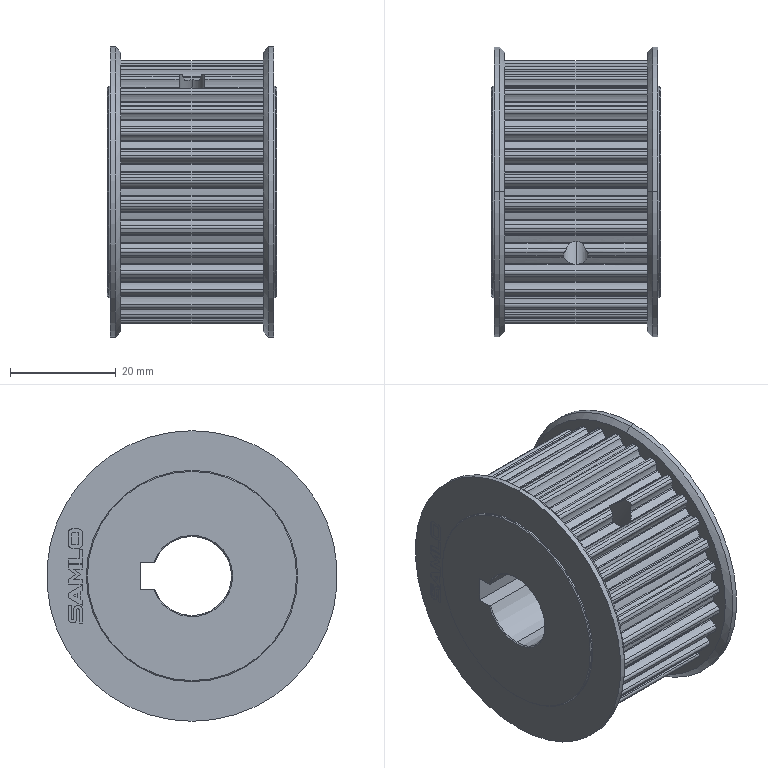Part | SolidWorks | features BaseBody 1 | 1 solid | 406 faces | box 32 x 55 x 55 mm | volume 52760 mm3 | cylinder 332 | plane 61 | cone 13 | commonest cylinder face diameters 1.1 x82 0.5 x81 6.55 x72 46.43 x35 49.97 x33 0.603 x4